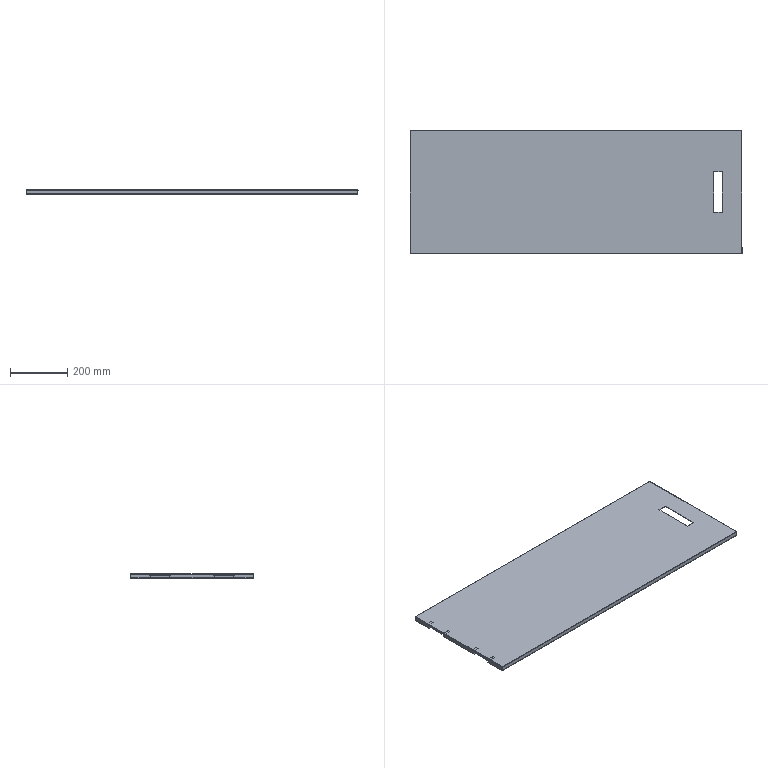Part | NX | features BREP 3 | 3 solids | 178 faces | box 1160 x 432 x 16.5 mm | volume 855904 mm3 | plane 114 | cylinder 48 | spline 16 | commonest cylinder face diameters 0.02 x18 3.02 x18 3.2 x12